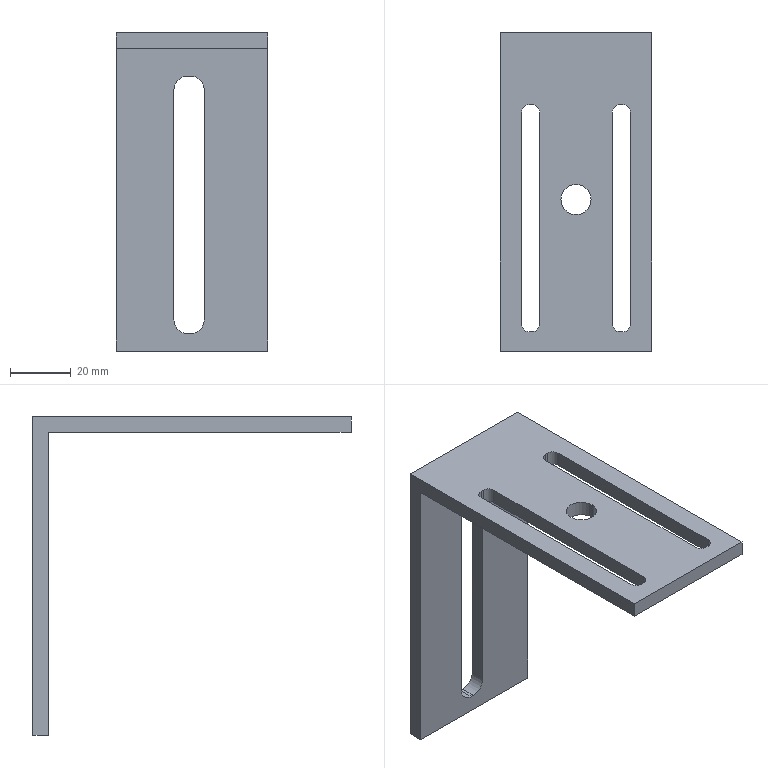Part | SolidWorks | features ICE 4, Extrusion 1 | 1 solid | 34 faces | box 50 x 105 x 105 mm | volume 42248 mm3 | plane 20 | cylinder 14 | commonest cylinder face diameters 5 x8 9 x4 10 x2
STEP:
#1=CARTESIAN_POINT('',(-5.,0.,0.));
#2=VERTEX_POINT('',#1);
#3=CARTESIAN_POINT('',(5.,0.,0.));
#4=VERTEX_POINT('',#3);
#5=CARTESIAN_POINT('',(0.,0.,0.));
#6=DIRECTION('',(0.,0.,1.));
#7=DIRECTION('',(1.,0.,0.));
#8=AXIS2_PLACEMENT_3D('',#5,#6,#7);
#9=CIRCLE('',#8,5.);
#10=EDGE_CURVE('',#2,#4,#9,.T.);
#11=ORIENTED_EDGE('',*,*,#10,.F.);
#12=CARTESIAN_POINT('',(-5.,0.,5.));
#13=VERTEX_POINT('',#12);
#14=CARTESIAN_POINT('',(-5.,0.,-5.));
#15=DIRECTION('',(0.,0.,1.));
#16=VECTOR('',#15,1000.);
#17=LINE('',#14,#16);
#18=EDGE_CURVE('',#2,#13,#17,.T.);
#19=ORIENTED_EDGE('',*,*,#18,.T.);
#20=CARTESIAN_POINT('',(5.,0.,5.));
#21=VERTEX_POINT('',#20);
#22=CARTESIAN_POINT('',(0.,0.,5.));
#23=DIRECTION('',(0.,0.,1.));
#24=DIRECTION('',(1.,0.,0.));
#25=AXIS2_PLACEMENT_3D('',#22,#23,#24);
#26=CIRCLE('',#25,5.);
#27=EDGE_CURVE('',#13,#21,#26,.T.);
#28=ORIENTED_EDGE('',*,*,#27,.T.);
#29=CARTESIAN_POINT('',(5.,0.,-5.));
#30=DIRECTION('',(0.,0.,1.));
#31=VECTOR('',#30,1000.);
#32=LINE('',#29,#31);
#33=EDGE_CURVE('',#4,#21,#32,.T.);
#34=ORIENTED_EDGE('',*,*,#33,.F.);
#35=EDGE_LOOP('',(#11,#19,#28,#34));
#36=FACE_OUTER_BOUND('',#35,.T.);
#37=CARTESIAN_POINT('',(0.,0.,-5.));
#38=DIRECTION('',(0.,0.,1.));
#39=DIRECTION('',(1.,0.,0.));
#40=AXIS2_PLACEMENT_3D('',#37,#38,#39);
#41=CYLINDRICAL_SURFACE('',#40,5.);
#42=ADVANCED_FACE('',(#36),#41,.F.);
#43=CARTESIAN_POINT('',(-25.,50.,0.));
#44=VERTEX_POINT('',#43);
#45=CARTESIAN_POINT('',(-25.,-50.,0.));
#46=VERTEX_POINT('',#45);
#47=CARTESIAN_POINT('',(-25.,-50.,0.));
#48=DIRECTION('',(0.,-1.,0.));
#49=VECTOR('',#48,1000.);
#50=LINE('',#47,#49);
#51=EDGE_CURVE('',#44,#46,#50,.T.);
#52=ORIENTED_EDGE('',*,*,#51,.T.);
#53=CARTESIAN_POINT('',(-25.,-50.,5.));
#54=VERTEX_POINT('',#53);
#55=CARTESIAN_POINT('',(-25.,-50.,5.));
#56=DIRECTION('',(0.,0.,-1.));
#57=VECTOR('',#56,1000.);
#58=LINE('',#55,#57);
#59=EDGE_CURVE('',#54,#46,#58,.T.);
#60=ORIENTED_EDGE('',*,*,#59,.F.);
#61=CARTESIAN_POINT('',(-25.,55.,5.));
#62=VERTEX_POINT('',#61);
#63=CARTESIAN_POINT('',(-25.,-50.,5.));
#64=DIRECTION('',(0.,-1.,0.));
#65=VECTOR('',#64,1000.);
#66=LINE('',#63,#65);
#67=EDGE_CURVE('',#62,#54,#66,.T.);
#68=ORIENTED_EDGE('',*,*,#67,.F.);
#69=CARTESIAN_POINT('',(-25.,55.,-100.));
#70=VERTEX_POINT('',#69);
#71=CARTESIAN_POINT('',(-25.,55.,5.));
#72=DIRECTION('',(0.,0.,-1.));
#73=VECTOR('',#72,1000.);
#74=LINE('',#71,#73);
#75=EDGE_CURVE('',#62,#70,#74,.T.);
#76=ORIENTED_EDGE('',*,*,#75,.T.);
#77=CARTESIAN_POINT('',(-25.,50.,-100.));
#78=VERTEX_POINT('',#77);
#79=CARTESIAN_POINT('',(-25.,50.,-100.));
#80=DIRECTION('',(0.,1.,0.));
#81=VECTOR('',#80,1000.);
#82=LINE('',#79,#81);
#83=EDGE_CURVE('',#78,#70,#82,.T.);
#84=ORIENTED_EDGE('',*,*,#83,.F.);
#85=CARTESIAN_POINT('',(-25.,50.,5.));
#86=DIRECTION('',(0.,0.,-1.));
#87=VECTOR('',#86,1000.);
#88=LINE('',#85,#87);
#89=EDGE_CURVE('',#44,#78,#88,.T.);
#90=ORIENTED_EDGE('',*,*,#89,.F.);
#91=EDGE_LOOP('',(#52,#60,#68,#76,#84,#90));
#92=FACE_OUTER_BOUND('',#91,.T.);
#93=CARTESIAN_POINT('',(-25.,-50.,5.));
#94=DIRECTION('',(1.,0.,0.));
#95=DIRECTION('',(0.,0.,-1.));
#96=AXIS2_PLACEMENT_3D('',#93,#94,#95);
#97=PLANE('',#96);
#98=ADVANCED_FACE('',(#92),#97,.F.);
#99=CARTESIAN_POINT('',(25.,-50.,0.));
#100=VERTEX_POINT('',#99);
#101=CARTESIAN_POINT('',(25.,-50.,0.));
#102=DIRECTION('',(1.,0.,0.));
#103=VECTOR('',#102,1000.);
#104=LINE('',#101,#103);
#105=EDGE_CURVE('',#46,#100,#104,.T.);
#106=ORIENTED_EDGE('',*,*,#105,.T.);
#107=CARTESIAN_POINT('',(25.,-50.,5.));
#108=VERTEX_POINT('',#107);
#109=CARTESIAN_POINT('',(25.,-50.,5.));
#110=DIRECTION('',(0.,0.,-1.));
#111=VECTOR('',#110,1000.);
#112=LINE('',#109,#111);
#113=EDGE_CURVE('',#108,#100,#112,.T.);
#114=ORIENTED_EDGE('',*,*,#113,.F.);
#115=CARTESIAN_POINT('',(25.,-50.,5.));
#116=DIRECTION('',(1.,0.,0.));
#117=VECTOR('',#116,1000.);
#118=LINE('',#115,#117);
#119=EDGE_CURVE('',#54,#108,#118,.T.);
#120=ORIENTED_EDGE('',*,*,#119,.F.);
#121=ORIENTED_EDGE('',*,*,#59,.T.);
#122=EDGE_LOOP('',(#106,#114,#120,#121));
#123=FACE_OUTER_BOUND('',#122,.T.);
#124=CARTESIAN_POINT('',(25.,-50.,5.));
#125=DIRECTION('',(0.,1.,0.));
#126=DIRECTION('',(-1.,0.,0.));
#127=AXIS2_PLACEMENT_3D('',#124,#125,#126);
#128=PLANE('',#127);
#129=ADVANCED_FACE('',(#123),#128,.F.);
#130=CARTESIAN_POINT('',(25.,50.,0.));
#131=VERTEX_POINT('',#130);
#132=CARTESIAN_POINT('',(25.,-50.,0.));
#133=DIRECTION('',(0.,1.,0.));
#134=VECTOR('',#133,1000.);
#135=LINE('',#132,#134);
#136=EDGE_CURVE('',#100,#131,#135,.T.);
#137=ORIENTED_EDGE('',*,*,#136,.T.);
#138=CARTESIAN_POINT('',(25.,50.,-100.));
#139=VERTEX_POINT('',#138);
#140=CARTESIAN_POINT('',(25.,50.,5.));
#141=DIRECTION('',(0.,0.,-1.));
#142=VECTOR('',#141,1000.);
#143=LINE('',#140,#142);
#144=EDGE_CURVE('',#131,#139,#143,.T.);
#145=ORIENTED_EDGE('',*,*,#144,.T.);
#146=CARTESIAN_POINT('',(25.,55.,-100.));
#147=VERTEX_POINT('',#146);
#148=CARTESIAN_POINT('',(25.,50.,-100.));
#149=DIRECTION('',(0.,-1.,0.));
#150=VECTOR('',#149,1000.);
#151=LINE('',#148,#150);
#152=EDGE_CURVE('',#147,#139,#151,.T.);
#153=ORIENTED_EDGE('',*,*,#152,.F.);
#154=CARTESIAN_POINT('',(25.,55.,5.));
#155=VERTEX_POINT('',#154);
#156=CARTESIAN_POINT('',(25.,55.,5.));
#157=DIRECTION('',(0.,0.,-1.));
#158=VECTOR('',#157,1000.);
#159=LINE('',#156,#158);
#160=EDGE_CURVE('',#155,#147,#159,.T.);
#161=ORIENTED_EDGE('',*,*,#160,.F.);
#162=CARTESIAN_POINT('',(25.,-50.,5.));
#163=DIRECTION('',(0.,1.,0.));
#164=VECTOR('',#163,1000.);
#165=LINE('',#162,#164);
#166=EDGE_CURVE('',#108,#155,#165,.T.);
#167=ORIENTED_EDGE('',*,*,#166,.F.);
#168=ORIENTED_EDGE('',*,*,#113,.T.);
#169=EDGE_LOOP('',(#137,#145,#153,#161,#167,#168));
#170=FACE_OUTER_BOUND('',#169,.T.);
#171=CARTESIAN_POINT('',(25.,-50.,5.));
#172=DIRECTION('',(-1.,0.,0.));
#173=DIRECTION('',(0.,0.,1.));
#174=AXIS2_PLACEMENT_3D('',#171,#172,#173);
#175=PLANE('',#174);
#176=ADVANCED_FACE('',(#170),#175,.F.);
#177=CARTESIAN_POINT('',(0.,0.,5.));
#178=DIRECTION('',(0.,0.,1.));
#179=DIRECTION('',(1.,0.,0.));
#180=AXIS2_PLACEMENT_3D('',#177,#178,#179);
#181=CIRCLE('',#180,5.);
#182=EDGE_CURVE('',#21,#13,#181,.T.);
#183=ORIENTED_EDGE('',*,*,#182,.F.);
#184=ORIENTED_EDGE('',*,*,#27,.F.);
#185=EDGE_LOOP('',(#183,#184));
#186=FACE_BOUND('',#185,.T.);
#187=CARTESIAN_POINT('',(-18.,-41.155,5.));
#188=VERTEX_POINT('',#187);
#189=CARTESIAN_POINT('',(-15.5,-43.655,5.));
#190=VERTEX_POINT('',#189);
#191=CARTESIAN_POINT('',(-15.5,-41.155,5.));
#192=DIRECTION('',(0.,0.,1.));
#193=DIRECTION('',(-1.,0.,0.));
#194=AXIS2_PLACEMENT_3D('',#191,#192,#193);
#195=CIRCLE('',#194,2.5);
#196=EDGE_CURVE('',#188,#190,#195,.T.);
#197=ORIENTED_EDGE('',*,*,#196,.F.);
#198=CARTESIAN_POINT('',(-18.,28.845,5.));
#199=VERTEX_POINT('',#198);
#200=CARTESIAN_POINT('',(-18.,-41.155,5.));
#201=DIRECTION('',(0.,-1.,0.));
#202=VECTOR('',#201,1000.);
#203=LINE('',#200,#202);
#204=EDGE_CURVE('',#199,#188,#203,.T.);
#205=ORIENTED_EDGE('',*,*,#204,.F.);
#206=CARTESIAN_POINT('',(-15.5,31.345,5.));
#207=VERTEX_POINT('',#206);
#208=CARTESIAN_POINT('',(-15.5,28.845,5.));
#209=DIRECTION('',(0.,0.,1.));
#210=DIRECTION('',(1.,0.,0.));
#211=AXIS2_PLACEMENT_3D('',#208,#209,#210);
#212=CIRCLE('',#211,2.5);
#213=EDGE_CURVE('',#207,#199,#212,.T.);
#214=ORIENTED_EDGE('',*,*,#213,.F.);
#215=CARTESIAN_POINT('',(-14.5,31.345,5.));
#216=VERTEX_POINT('',#215);
#217=CARTESIAN_POINT('',(-14.5,31.345,5.));
#218=DIRECTION('',(-1.,0.,0.));
#219=VECTOR('',#218,1000.);
#220=LINE('',#217,#219);
#221=EDGE_CURVE('',#216,#207,#220,.T.);
#222=ORIENTED_EDGE('',*,*,#221,.F.);
#223=CARTESIAN_POINT('',(-12.,28.845,5.));
#224=VERTEX_POINT('',#223);
#225=CARTESIAN_POINT('',(-14.5,28.845,5.));
#226=DIRECTION('',(0.,0.,1.));
#227=DIRECTION('',(1.,0.,0.));
#228=AXIS2_PLACEMENT_3D('',#225,#226,#227);
#229=CIRCLE('',#228,2.5);
#230=EDGE_CURVE('',#224,#216,#229,.T.);
#231=ORIENTED_EDGE('',*,*,#230,.F.);
#232=CARTESIAN_POINT('',(-12.,-41.155,5.));
#233=VERTEX_POINT('',#232);
#234=CARTESIAN_POINT('',(-12.,-41.155,5.));
#235=DIRECTION('',(0.,1.,0.));
#236=VECTOR('',#235,1000.);
#237=LINE('',#234,#236);
#238=EDGE_CURVE('',#233,#224,#237,.T.);
#239=ORIENTED_EDGE('',*,*,#238,.F.);
#240=CARTESIAN_POINT('',(-14.5,-43.655,5.));
#241=VERTEX_POINT('',#240);
#242=CARTESIAN_POINT('',(-14.5,-41.155,5.));
#243=DIRECTION('',(0.,0.,1.));
#244=DIRECTION('',(1.,0.,0.));
#245=AXIS2_PLACEMENT_3D('',#242,#243,#244);
#246=CIRCLE('',#245,2.5);
#247=EDGE_CURVE('',#241,#233,#246,.T.);
#248=ORIENTED_EDGE('',*,*,#247,.F.);
#249=CARTESIAN_POINT('',(-14.5,-43.655,5.));
#250=DIRECTION('',(1.,0.,0.));
#251=VECTOR('',#250,1000.);
#252=LINE('',#249,#251);
#253=EDGE_CURVE('',#190,#241,#252,.T.);
#254=ORIENTED_EDGE('',*,*,#253,.F.);
#255=EDGE_LOOP('',(#197,#205,#214,#222,#231,#239,#248,#254));
#256=FACE_BOUND('',#255,.T.);
#257=CARTESIAN_POINT('',(14.5,31.345,5.));
#258=VERTEX_POINT('',#257);
#259=CARTESIAN_POINT('',(12.,28.845,5.));
#260=VERTEX_POINT('',#259);
#261=CARTESIAN_POINT('',(14.5,28.845,5.));
#262=DIRECTION('',(0.,0.,1.));
#263=DIRECTION('',(1.,0.,0.));
#264=AXIS2_PLACEMENT_3D('',#261,#262,#263);
#265=CIRCLE('',#264,2.5);
#266=EDGE_CURVE('',#258,#260,#265,.T.);
#267=ORIENTED_EDGE('',*,*,#266,.F.);
#268=CARTESIAN_POINT('',(15.5,31.345,5.));
#269=VERTEX_POINT('',#268);
#270=CARTESIAN_POINT('',(15.5,31.345,5.));
#271=DIRECTION('',(-1.,0.,0.));
#272=VECTOR('',#271,1000.);
#273=LINE('',#270,#272);
#274=EDGE_CURVE('',#269,#258,#273,.T.);
#275=ORIENTED_EDGE('',*,*,#274,.F.);
#276=CARTESIAN_POINT('',(18.,28.845,5.));
#277=VERTEX_POINT('',#276);
#278=CARTESIAN_POINT('',(15.5,28.845,5.));
#279=DIRECTION('',(0.,0.,1.));
#280=DIRECTION('',(1.,0.,0.));
#281=AXIS2_PLACEMENT_3D('',#278,#279,#280);
#282=CIRCLE('',#281,2.5);
#283=EDGE_CURVE('',#277,#269,#282,.T.);
#284=ORIENTED_EDGE('',*,*,#283,.F.);
#285=CARTESIAN_POINT('',(18.,-41.155,5.));
#286=VERTEX_POINT('',#285);
#287=CARTESIAN_POINT('',(18.,-41.155,5.));
#288=DIRECTION('',(0.,1.,0.));
#289=VECTOR('',#288,1000.);
#290=LINE('',#287,#289);
#291=EDGE_CURVE('',#286,#277,#290,.T.);
#292=ORIENTED_EDGE('',*,*,#291,.F.);
#293=CARTESIAN_POINT('',(15.5,-43.655,5.));
#294=VERTEX_POINT('',#293);
#295=CARTESIAN_POINT('',(15.5,-41.155,5.));
#296=DIRECTION('',(0.,0.,1.));
#297=DIRECTION('',(1.,0.,0.));
#298=AXIS2_PLACEMENT_3D('',#295,#296,#297);
#299=CIRCLE('',#298,2.5);
#300=EDGE_CURVE('',#294,#286,#299,.T.);
#301=ORIENTED_EDGE('',*,*,#300,.F.);
#302=CARTESIAN_POINT('',(14.5,-43.655,5.));
#303=VERTEX_POINT('',#302);
#304=CARTESIAN_POINT('',(15.5,-43.655,5.));
#305=DIRECTION('',(1.,0.,0.));
#306=VECTOR('',#305,1000.);
#307=LINE('',#304,#306);
#308=EDGE_CURVE('',#303,#294,#307,.T.);
#309=ORIENTED_EDGE('',*,*,#308,.F.);
#310=CARTESIAN_POINT('',(12.,-41.155,5.));
#311=VERTEX_POINT('',#310);
#312=CARTESIAN_POINT('',(14.5,-41.155,5.));
#313=DIRECTION('',(0.,0.,1.));
#314=DIRECTION('',(-1.,0.,0.));
#315=AXIS2_PLACEMENT_3D('',#312,#313,#314);
#316=CIRCLE('',#315,2.5);
#317=EDGE_CURVE('',#311,#303,#316,.T.);
#318=ORIENTED_EDGE('',*,*,#317,.F.);
#319=CARTESIAN_POINT('',(12.,-41.155,5.));
#320=DIRECTION('',(0.,-1.,0.));
#321=VECTOR('',#320,1000.);
#322=LINE('',#319,#321);
#323=EDGE_CURVE('',#260,#311,#322,.T.);
#324=ORIENTED_EDGE('',*,*,#323,.F.);
#325=EDGE_LOOP('',(#267,#275,#284,#292,#301,#309,#318,#324));
#326=FACE_BOUND('',#325,.T.);
#327=ORIENTED_EDGE('',*,*,#67,.T.);
#328=ORIENTED_EDGE('',*,*,#119,.T.);
#329=ORIENTED_EDGE('',*,*,#166,.T.);
#330=CARTESIAN_POINT('',(-25.,55.,5.));
#331=DIRECTION('',(1.,0.,0.));
#332=VECTOR('',#331,1000.);
#333=LINE('',#330,#332);
#334=EDGE_CURVE('',#62,#155,#333,.T.);
#335=ORIENTED_EDGE('',*,*,#334,.F.);
#336=EDGE_LOOP('',(#327,#328,#329,#335));
#337=FACE_OUTER_BOUND('',#336,.T.);
#338=CARTESIAN_POINT('',(-25.,50.,5.));
#339=DIRECTION('',(0.,0.,1.));
#340=DIRECTION('',(1.,0.,0.));
#341=AXIS2_PLACEMENT_3D('',#338,#339,#340);
#342=PLANE('',#341);
#343=ADVANCED_FACE('',(#186,#256,#326,#337),#342,.T.);
#344=CARTESIAN_POINT('',(0.,0.,0.));
#345=DIRECTION('',(0.,0.,1.));
#346=DIRECTION('',(1.,0.,0.));
#347=AXIS2_PLACEMENT_3D('',#344,#345,#346);
#348=CIRCLE('',#347,5.);
#349=EDGE_CURVE('',#4,#2,#348,.T.);
#350=ORIENTED_EDGE('',*,*,#349,.T.);
#351=ORIENTED_EDGE('',*,*,#10,.T.);
#352=EDGE_LOOP('',(#350,#351));
#353=FACE_BOUND('',#352,.T.);
#354=CARTESIAN_POINT('',(-18.,28.845,0.));
#355=VERTEX_POINT('',#354);
#356=CARTESIAN_POINT('',(-18.,-41.155,0.));
#357=VERTEX_POINT('',#356);
#358=CARTESIAN_POINT('',(-18.,50.,0.));
#359=DIRECTION('',(0.,-1.,0.));
#360=VECTOR('',#359,1000.);
#361=LINE('',#358,#360);
#362=EDGE_CURVE('',#355,#357,#361,.T.);
#363=ORIENTED_EDGE('',*,*,#362,.T.);
#364=CARTESIAN_POINT('',(-15.5,-43.655,0.));
#365=VERTEX_POINT('',#364);
#366=CARTESIAN_POINT('',(-15.5,-41.155,0.));
#367=DIRECTION('',(0.,0.,1.));
#368=DIRECTION('',(1.,0.,0.));
#369=AXIS2_PLACEMENT_3D('',#366,#367,#368);
#370=CIRCLE('',#369,2.5);
#371=EDGE_CURVE('',#357,#365,#370,.T.);
#372=ORIENTED_EDGE('',*,*,#371,.T.);
#373=CARTESIAN_POINT('',(-14.5,-43.655,0.));
#374=VERTEX_POINT('',#373);
#375=CARTESIAN_POINT('',(-25.,-43.655,0.));
#376=DIRECTION('',(1.,0.,0.));
#377=VECTOR('',#376,1000.);
#378=LINE('',#375,#377);
#379=EDGE_CURVE('',#365,#374,#378,.T.);
#380=ORIENTED_EDGE('',*,*,#379,.T.);
#381=CARTESIAN_POINT('',(-12.,-41.155,0.));
#382=VERTEX_POINT('',#381);
#383=CARTESIAN_POINT('',(-14.5,-41.155,0.));
#384=DIRECTION('',(0.,0.,1.));
#385=DIRECTION('',(1.,0.,0.));
#386=AXIS2_PLACEMENT_3D('',#383,#384,#385);
#387=CIRCLE('',#386,2.5);
#388=EDGE_CURVE('',#374,#382,#387,.T.);
#389=ORIENTED_EDGE('',*,*,#388,.T.);
#390=CARTESIAN_POINT('',(-12.,28.845,0.));
#391=VERTEX_POINT('',#390);
#392=CARTESIAN_POINT('',(-12.,50.,0.));
#393=DIRECTION('',(0.,1.,0.));
#394=VECTOR('',#393,1000.);
#395=LINE('',#392,#394);
#396=EDGE_CURVE('',#382,#391,#395,.T.);
#397=ORIENTED_EDGE('',*,*,#396,.T.);
#398=CARTESIAN_POINT('',(-14.5,31.345,0.));
#399=VERTEX_POINT('',#398);
#400=CARTESIAN_POINT('',(-14.5,28.845,0.));
#401=DIRECTION('',(0.,0.,1.));
#402=DIRECTION('',(1.,0.,0.));
#403=AXIS2_PLACEMENT_3D('',#400,#401,#402);
#404=CIRCLE('',#403,2.5);
#405=EDGE_CURVE('',#391,#399,#404,.T.);
#406=ORIENTED_EDGE('',*,*,#405,.T.);
#407=CARTESIAN_POINT('',(-15.5,31.345,0.));
#408=VERTEX_POINT('',#407);
#409=CARTESIAN_POINT('',(-25.,31.345,0.));
#410=DIRECTION('',(-1.,0.,0.));
#411=VECTOR('',#410,1000.);
#412=LINE('',#409,#411);
#413=EDGE_CURVE('',#399,#408,#412,.T.);
#414=ORIENTED_EDGE('',*,*,#413,.T.);
#415=CARTESIAN_POINT('',(-15.5,28.845,0.));
#416=DIRECTION('',(0.,0.,1.));
#417=DIRECTION('',(1.,0.,0.));
#418=AXIS2_PLACEMENT_3D('',#415,#416,#417);
#419=CIRCLE('',#418,2.5);
#420=EDGE_CURVE('',#408,#355,#419,.T.);
#421=ORIENTED_EDGE('',*,*,#420,.T.);
#422=EDGE_LOOP('',(#363,#372,#380,#389,#397,#406,#414,#421));
#423=FACE_BOUND('',#422,.T.);
#424=CARTESIAN_POINT('',(15.5,31.345,0.));
#425=VERTEX_POINT('',#424);
#426=CARTESIAN_POINT('',(14.5,31.345,0.));
#427=VERTEX_POINT('',#426);
#428=CARTESIAN_POINT('',(-25.,31.345,0.));
#429=DIRECTION('',(-1.,0.,0.));
#430=VECTOR('',#429,1000.);
#431=LINE('',#428,#430);
#432=EDGE_CURVE('',#425,#427,#431,.T.);
#433=ORIENTED_EDGE('',*,*,#432,.T.);
#434=CARTESIAN_POINT('',(12.,28.845,0.));
#435=VERTEX_POINT('',#434);
#436=CARTESIAN_POINT('',(14.5,28.845,0.));
#437=DIRECTION('',(0.,0.,1.));
#438=DIRECTION('',(1.,0.,0.));
#439=AXIS2_PLACEMENT_3D('',#436,#437,#438);
#440=CIRCLE('',#439,2.5);
#441=EDGE_CURVE('',#427,#435,#440,.T.);
#442=ORIENTED_EDGE('',*,*,#441,.T.);
#443=CARTESIAN_POINT('',(12.,-41.155,0.));
#444=VERTEX_POINT('',#443);
#445=CARTESIAN_POINT('',(12.,50.,0.));
#446=DIRECTION('',(0.,-1.,0.));
#447=VECTOR('',#446,1000.);
#448=LINE('',#445,#447);
#449=EDGE_CURVE('',#435,#444,#448,.T.);
#450=ORIENTED_EDGE('',*,*,#449,.T.);
#451=CARTESIAN_POINT('',(14.5,-43.655,0.));
#452=VERTEX_POINT('',#451);
#453=CARTESIAN_POINT('',(14.5,-41.155,0.));
#454=DIRECTION('',(0.,0.,1.));
#455=DIRECTION('',(1.,0.,0.));
#456=AXIS2_PLACEMENT_3D('',#453,#454,#455);
#457=CIRCLE('',#456,2.5);
#458=EDGE_CURVE('',#444,#452,#457,.T.);
#459=ORIENTED_EDGE('',*,*,#458,.T.);
#460=CARTESIAN_POINT('',(15.5,-43.655,0.));
#461=VERTEX_POINT('',#460);
#462=CARTESIAN_POINT('',(-25.,-43.655,0.));
#463=DIRECTION('',(1.,0.,0.));
#464=VECTOR('',#463,1000.);
#465=LINE('',#462,#464);
#466=EDGE_CURVE('',#452,#461,#465,.T.);
#467=ORIENTED_EDGE('',*,*,#466,.T.);
#468=CARTESIAN_POINT('',(18.,-41.155,0.));
#469=VERTEX_POINT('',#468);
#470=CARTESIAN_POINT('',(15.5,-41.155,0.));
#471=DIRECTION('',(0.,0.,1.));
#472=DIRECTION('',(1.,0.,0.));
#473=AXIS2_PLACEMENT_3D('',#470,#471,#472);
#474=CIRCLE('',#473,2.5);
#475=EDGE_CURVE('',#461,#469,#474,.T.);
#476=ORIENTED_EDGE('',*,*,#475,.T.);
#477=CARTESIAN_POINT('',(18.,28.845,0.));
#478=VERTEX_POINT('',#477);
#479=CARTESIAN_POINT('',(18.,50.,0.));
#480=DIRECTION('',(0.,1.,0.));
#481=VECTOR('',#480,1000.);
#482=LINE('',#479,#481);
#483=EDGE_CURVE('',#469,#478,#482,.T.);
#484=ORIENTED_EDGE('',*,*,#483,.T.);
#485=CARTESIAN_POINT('',(15.5,28.845,0.));
#486=DIRECTION('',(0.,0.,1.));
#487=DIRECTION('',(1.,0.,0.));
#488=AXIS2_PLACEMENT_3D('',#485,#486,#487);
#489=CIRCLE('',#488,2.5);
#490=EDGE_CURVE('',#478,#425,#489,.T.);
#491=ORIENTED_EDGE('',*,*,#490,.T.);
#492=EDGE_LOOP('',(#433,#442,#450,#459,#467,#476,#484,#491));
#493=FACE_BOUND('',#492,.T.);
#494=ORIENTED_EDGE('',*,*,#51,.F.);
#495=CARTESIAN_POINT('',(25.,50.,0.));
#496=DIRECTION('',(-1.,0.,0.));
#497=VECTOR('',#496,1000.);
#498=LINE('',#495,#497);
#499=EDGE_CURVE('',#131,#44,#498,.T.);
#500=ORIENTED_EDGE('',*,*,#499,.F.);
#501=ORIENTED_EDGE('',*,*,#136,.F.);
#502=ORIENTED_EDGE('',*,*,#105,.F.);
#503=EDGE_LOOP('',(#494,#500,#501,#502));
#504=FACE_OUTER_BOUND('',#503,.T.);
#505=CARTESIAN_POINT('',(-25.,50.,0.));
#506=DIRECTION('',(0.,0.,1.));
#507=DIRECTION('',(1.,0.,0.));
#508=AXIS2_PLACEMENT_3D('',#505,#506,#507);
#509=PLANE('',#508);
#510=ADVANCED_FACE('',(#353,#423,#493,#504),#509,.F.);
#511=CARTESIAN_POINT('',(14.5,31.345,-5.));
#512=DIRECTION('',(0.,0.,1.));
#513=VECTOR('',#512,1000.);
#514=LINE('',#511,#513);
#515=EDGE_CURVE('',#427,#258,#514,.T.);
#516=ORIENTED_EDGE('',*,*,#515,.T.);
#517=ORIENTED_EDGE('',*,*,#266,.T.);
#518=CARTESIAN_POINT('',(12.,28.845,-5.));
#519=DIRECTION('',(0.,0.,1.));
#520=VECTOR('',#519,1000.);
#521=LINE('',#518,#520);
#522=EDGE_CURVE('',#435,#260,#521,.T.);
#523=ORIENTED_EDGE('',*,*,#522,.F.);
#524=ORIENTED_EDGE('',*,*,#441,.F.);
#525=EDGE_LOOP('',(#516,#517,#523,#524));
#526=FACE_OUTER_BOUND('',#525,.T.);
#527=CARTESIAN_POINT('',(14.5,28.845,-5.));
#528=DIRECTION('',(0.,0.,1.));
#529=DIRECTION('',(1.,0.,0.));
#530=AXIS2_PLACEMENT_3D('',#527,#528,#529);
#531=CYLINDRICAL_SURFACE('',#530,2.5);
#532=ADVANCED_FACE('',(#526),#531,.F.);
#533=CARTESIAN_POINT('',(15.5,31.345,-5.));
#534=DIRECTION('',(0.,0.,1.));
#535=VECTOR('',#534,1000.);
#536=LINE('',#533,#535);
#537=EDGE_CURVE('',#425,#269,#536,.T.);
#538=ORIENTED_EDGE('',*,*,#537,.T.);
#539=ORIENTED_EDGE('',*,*,#274,.T.);
#540=ORIENTED_EDGE('',*,*,#515,.F.);
#541=ORIENTED_EDGE('',*,*,#432,.F.);
#542=EDGE_LOOP('',(#538,#539,#540,#541));
#543=FACE_OUTER_BOUND('',#542,.T.);
#544=CARTESIAN_POINT('',(15.5,31.345,-5.));
#545=DIRECTION('',(0.,1.,0.));
#546=DIRECTION('',(0.,0.,1.));
#547=AXIS2_PLACEMENT_3D('',#544,#545,#546);
#548=PLANE('',#547);
#549=ADVANCED_FACE('',(#543),#548,.F.);
#550=CARTESIAN_POINT('',(18.,28.845,-5.));
#551=DIRECTION('',(0.,0.,1.));
#552=VECTOR('',#551,1000.);
#553=LINE('',#550,#552);
#554=EDGE_CURVE('',#478,#277,#553,.T.);
#555=ORIENTED_EDGE('',*,*,#554,.T.);
#556=ORIENTED_EDGE('',*,*,#283,.T.);
#557=ORIENTED_EDGE('',*,*,#537,.F.);
#558=ORIENTED_EDGE('',*,*,#490,.F.);
#559=EDGE_LOOP('',(#555,#556,#557,#558));
#560=FACE_OUTER_BOUND('',#559,.T.);
#561=CARTESIAN_POINT('',(15.5,28.845,-5.));
#562=DIRECTION('',(0.,0.,1.));
#563=DIRECTION('',(1.,0.,0.));
#564=AXIS2_PLACEMENT_3D('',#561,#562,#563);
#565=CYLINDRICAL_SURFACE('',#564,2.5);
#566=ADVANCED_FACE('',(#560),#565,.F.);
#567=CARTESIAN_POINT('',(18.,-41.155,-5.));
#568=DIRECTION('',(0.,0.,1.));
#569=VECTOR('',#568,1000.);
#570=LINE('',#567,#569);
#571=EDGE_CURVE('',#469,#286,#570,.T.);
#572=ORIENTED_EDGE('',*,*,#571,.T.);
#573=ORIENTED_EDGE('',*,*,#291,.T.);
#574=ORIENTED_EDGE('',*,*,#554,.F.);
#575=ORIENTED_EDGE('',*,*,#483,.F.);
#576=EDGE_LOOP('',(#572,#573,#574,#575));
#577=FACE_OUTER_BOUND('',#576,.T.);
#578=CARTESIAN_POINT('',(18.,-41.155,-5.));
#579=DIRECTION('',(1.,0.,0.));
#580=DIRECTION('',(0.,0.,-1.));
#581=AXIS2_PLACEMENT_3D('',#578,#579,#580);
#582=PLANE('',#581);
#583=ADVANCED_FACE('',(#577),#582,.F.);
#584=CARTESIAN_POINT('',(15.5,-43.655,-5.));
#585=DIRECTION('',(0.,0.,1.));
#586=VECTOR('',#585,1000.);
#587=LINE('',#584,#586);
#588=EDGE_CURVE('',#461,#294,#587,.T.);
#589=ORIENTED_EDGE('',*,*,#588,.T.);
#590=ORIENTED_EDGE('',*,*,#300,.T.);
#591=ORIENTED_EDGE('',*,*,#571,.F.);
#592=ORIENTED_EDGE('',*,*,#475,.F.);
#593=EDGE_LOOP('',(#589,#590,#591,#592));
#594=FACE_OUTER_BOUND('',#593,.T.);
#595=CARTESIAN_POINT('',(15.5,-41.155,-5.));
#596=DIRECTION('',(0.,0.,1.));
#597=DIRECTION('',(1.,0.,0.));
#598=AXIS2_PLACEMENT_3D('',#595,#596,#597);
#599=CYLINDRICAL_SURFACE('',#598,2.5);
#600=ADVANCED_FACE('',(#594),#599,.F.);
#601=CARTESIAN_POINT('',(14.5,-43.655,-5.));
#602=DIRECTION('',(0.,0.,1.));
#603=VECTOR('',#602,1000.);
#604=LINE('',#601,#603);
#605=EDGE_CURVE('',#452,#303,#604,.T.);
#606=ORIENTED_EDGE('',*,*,#605,.T.);
#607=ORIENTED_EDGE('',*,*,#308,.T.);
#608=ORIENTED_EDGE('',*,*,#588,.F.);
#609=ORIENTED_EDGE('',*,*,#466,.F.);
#610=EDGE_LOOP('',(#606,#607,#608,#609));
#611=FACE_OUTER_BOUND('',#610,.T.);
#612=CARTESIAN_POINT('',(15.5,-43.655,-5.));
#613=DIRECTION('',(0.,-1.,0.));
#614=DIRECTION('',(0.,0.,-1.));
#615=AXIS2_PLACEMENT_3D('',#612,#613,#614);
#616=PLANE('',#615);
#617=ADVANCED_FACE('',(#611),#616,.F.);
#618=CARTESIAN_POINT('',(12.,-41.155,-5.));
#619=DIRECTION('',(0.,0.,1.));
#620=VECTOR('',#619,1000.);
#621=LINE('',#618,#620);
#622=EDGE_CURVE('',#444,#311,#621,.T.);
#623=ORIENTED_EDGE('',*,*,#622,.T.);
#624=ORIENTED_EDGE('',*,*,#317,.T.);
#625=ORIENTED_EDGE('',*,*,#605,.F.);
#626=ORIENTED_EDGE('',*,*,#458,.F.);
#627=EDGE_LOOP('',(#623,#624,#625,#626));
#628=FACE_OUTER_BOUND('',#627,.T.);
#629=CARTESIAN_POINT('',(14.5,-41.155,-5.));
#630=DIRECTION('',(0.,0.,1.));
#631=DIRECTION('',(1.,0.,0.));
#632=AXIS2_PLACEMENT_3D('',#629,#630,#631);
#633=CYLINDRICAL_SURFACE('',#632,2.5);
#634=ADVANCED_FACE('',(#628),#633,.F.);
#635=ORIENTED_EDGE('',*,*,#522,.T.);
#636=ORIENTED_EDGE('',*,*,#323,.T.);
#637=ORIENTED_EDGE('',*,*,#622,.F.);
#638=ORIENTED_EDGE('',*,*,#449,.F.);
#639=EDGE_LOOP('',(#635,#636,#637,#638));
#640=FACE_OUTER_BOUND('',#639,.T.);
#641=CARTESIAN_POINT('',(12.,-41.155,-5.));
#642=DIRECTION('',(-1.,0.,0.));
#643=DIRECTION('',(0.,0.,1.));
#644=AXIS2_PLACEMENT_3D('',#641,#642,#643);
#645=PLANE('',#644);
#646=ADVANCED_FACE('',(#640),#645,.F.);
#647=CARTESIAN_POINT('',(-18.,-41.155,-5.));
#648=DIRECTION('',(0.,0.,1.));
#649=VECTOR('',#648,1000.);
#650=LINE('',#647,#649);
#651=EDGE_CURVE('',#357,#188,#650,.T.);
#652=ORIENTED_EDGE('',*,*,#651,.T.);
#653=ORIENTED_EDGE('',*,*,#196,.T.);
#654=CARTESIAN_POINT('',(-15.5,-43.655,-5.));
#655=DIRECTION('',(0.,0.,1.));
#656=VECTOR('',#655,1000.);
#657=LINE('',#654,#656);
#658=EDGE_CURVE('',#365,#190,#657,.T.);
#659=ORIENTED_EDGE('',*,*,#658,.F.);
#660=ORIENTED_EDGE('',*,*,#371,.F.);
#661=EDGE_LOOP('',(#652,#653,#659,#660));
#662=FACE_OUTER_BOUND('',#661,.T.);
#663=CARTESIAN_POINT('',(-15.5,-41.155,-5.));
#664=DIRECTION('',(0.,0.,1.));
#665=DIRECTION('',(1.,0.,0.));
#666=AXIS2_PLACEMENT_3D('',#663,#664,#665);
#667=CYLINDRICAL_SURFACE('',#666,2.5);
#668=ADVANCED_FACE('',(#662),#667,.F.);
#669=CARTESIAN_POINT('',(-18.,28.845,-5.));
#670=DIRECTION('',(0.,0.,1.));
#671=VECTOR('',#670,1000.);
#672=LINE('',#669,#671);
#673=EDGE_CURVE('',#355,#199,#672,.T.);
#674=ORIENTED_EDGE('',*,*,#673,.T.);
#675=ORIENTED_EDGE('',*,*,#204,.T.);
#676=ORIENTED_EDGE('',*,*,#651,.F.);
#677=ORIENTED_EDGE('',*,*,#362,.F.);
#678=EDGE_LOOP('',(#674,#675,#676,#677));
#679=FACE_OUTER_BOUND('',#678,.T.);
#680=CARTESIAN_POINT('',(-18.,-41.155,-5.));
#681=DIRECTION('',(-1.,0.,0.));
#682=DIRECTION('',(0.,0.,1.));
#683=AXIS2_PLACEMENT_3D('',#680,#681,#682);
#684=PLANE('',#683);
#685=ADVANCED_FACE('',(#679),#684,.F.);
#686=CARTESIAN_POINT('',(-15.5,31.345,-5.));
#687=DIRECTION('',(0.,0.,1.));
#688=VECTOR('',#687,1000.);
#689=LINE('',#686,#688);
#690=EDGE_CURVE('',#408,#207,#689,.T.);
#691=ORIENTED_EDGE('',*,*,#690,.T.);
#692=ORIENTED_EDGE('',*,*,#213,.T.);
#693=ORIENTED_EDGE('',*,*,#673,.F.);
#694=ORIENTED_EDGE('',*,*,#420,.F.);
#695=EDGE_LOOP('',(#691,#692,#693,#694));
#696=FACE_OUTER_BOUND('',#695,.T.);
#697=CARTESIAN_POINT('',(-15.5,28.845,-5.));
#698=DIRECTION('',(0.,0.,1.));
#699=DIRECTION('',(1.,0.,0.));
#700=AXIS2_PLACEMENT_3D('',#697,#698,#699);
#701=CYLINDRICAL_SURFACE('',#700,2.5);
#702=ADVANCED_FACE('',(#696),#701,.F.);
#703=CARTESIAN_POINT('',(-14.5,31.345,-5.));
#704=DIRECTION('',(0.,0.,1.));
#705=VECTOR('',#704,1000.);
#706=LINE('',#703,#705);
#707=EDGE_CURVE('',#399,#216,#706,.T.);
#708=ORIENTED_EDGE('',*,*,#707,.T.);
#709=ORIENTED_EDGE('',*,*,#221,.T.);
#710=ORIENTED_EDGE('',*,*,#690,.F.);
#711=ORIENTED_EDGE('',*,*,#413,.F.);
#712=EDGE_LOOP('',(#708,#709,#710,#711));
#713=FACE_OUTER_BOUND('',#712,.T.);
#714=CARTESIAN_POINT('',(-14.5,31.345,-5.));
#715=DIRECTION('',(0.,1.,0.));
#716=DIRECTION('',(0.,0.,1.));
#717=AXIS2_PLACEMENT_3D('',#714,#715,#716);
#718=PLANE('',#717);
#719=ADVANCED_FACE('',(#713),#718,.F.);
#720=CARTESIAN_POINT('',(-12.,28.845,-5.));
#721=DIRECTION('',(0.,0.,1.));
#722=VECTOR('',#721,1000.);
#723=LINE('',#720,#722);
#724=EDGE_CURVE('',#391,#224,#723,.T.);
#725=ORIENTED_EDGE('',*,*,#724,.T.);
#726=ORIENTED_EDGE('',*,*,#230,.T.);
#727=ORIENTED_EDGE('',*,*,#707,.F.);
#728=ORIENTED_EDGE('',*,*,#405,.F.);
#729=EDGE_LOOP('',(#725,#726,#727,#728));
#730=FACE_OUTER_BOUND('',#729,.T.);
#731=CARTESIAN_POINT('',(-14.5,28.845,-5.));
#732=DIRECTION('',(0.,0.,1.));
#733=DIRECTION('',(1.,0.,0.));
#734=AXIS2_PLACEMENT_3D('',#731,#732,#733);
#735=CYLINDRICAL_SURFACE('',#734,2.5);
#736=ADVANCED_FACE('',(#730),#735,.F.);
#737=CARTESIAN_POINT('',(-12.,-41.155,-5.));
#738=DIRECTION('',(0.,0.,1.));
#739=VECTOR('',#738,1000.);
#740=LINE('',#737,#739);
#741=EDGE_CURVE('',#382,#233,#740,.T.);
#742=ORIENTED_EDGE('',*,*,#741,.T.);
#743=ORIENTED_EDGE('',*,*,#238,.T.);
#744=ORIENTED_EDGE('',*,*,#724,.F.);
#745=ORIENTED_EDGE('',*,*,#396,.F.);
#746=EDGE_LOOP('',(#742,#743,#744,#745));
#747=FACE_OUTER_BOUND('',#746,.T.);
#748=CARTESIAN_POINT('',(-12.,-41.155,-5.));
#749=DIRECTION('',(1.,0.,0.));
#750=DIRECTION('',(0.,0.,-1.));
#751=AXIS2_PLACEMENT_3D('',#748,#749,#750);
#752=PLANE('',#751);
#753=ADVANCED_FACE('',(#747),#752,.F.);
#754=CARTESIAN_POINT('',(-14.5,-43.655,-5.));
#755=DIRECTION('',(0.,0.,1.));
#756=VECTOR('',#755,1000.);
#757=LINE('',#754,#756);
#758=EDGE_CURVE('',#374,#241,#757,.T.);
#759=ORIENTED_EDGE('',*,*,#758,.T.);
#760=ORIENTED_EDGE('',*,*,#247,.T.);
#761=ORIENTED_EDGE('',*,*,#741,.F.);
#762=ORIENTED_EDGE('',*,*,#388,.F.);
#763=EDGE_LOOP('',(#759,#760,#761,#762));
#764=FACE_OUTER_BOUND('',#763,.T.);
#765=CARTESIAN_POINT('',(-14.5,-41.155,-5.));
#766=DIRECTION('',(0.,0.,1.));
#767=DIRECTION('',(1.,0.,0.));
#768=AXIS2_PLACEMENT_3D('',#765,#766,#767);
#769=CYLINDRICAL_SURFACE('',#768,2.5);
#770=ADVANCED_FACE('',(#764),#769,.F.);
#771=ORIENTED_EDGE('',*,*,#658,.T.);
#772=ORIENTED_EDGE('',*,*,#253,.T.);
#773=ORIENTED_EDGE('',*,*,#758,.F.);
#774=ORIENTED_EDGE('',*,*,#379,.F.);
#775=EDGE_LOOP('',(#771,#772,#773,#774));
#776=FACE_OUTER_BOUND('',#775,.T.);
#777=CARTESIAN_POINT('',(-14.5,-43.655,-5.));
#778=DIRECTION('',(0.,-1.,0.));
#779=DIRECTION('',(0.,0.,-1.));
#780=AXIS2_PLACEMENT_3D('',#777,#778,#779);
#781=PLANE('',#780);
#782=ADVANCED_FACE('',(#776),#781,.F.);
#783=ORIENTED_EDGE('',*,*,#18,.F.);
#784=ORIENTED_EDGE('',*,*,#349,.F.);
#785=ORIENTED_EDGE('',*,*,#33,.T.);
#786=ORIENTED_EDGE('',*,*,#182,.T.);
#787=EDGE_LOOP('',(#783,#784,#785,#786));
#788=FACE_OUTER_BOUND('',#787,.T.);
#789=CARTESIAN_POINT('',(0.,0.,-5.));
#790=DIRECTION('',(0.,0.,1.));
#791=DIRECTION('',(1.,0.,0.));
#792=AXIS2_PLACEMENT_3D('',#789,#790,#791);
#793=CYLINDRICAL_SURFACE('',#792,5.);
#794=ADVANCED_FACE('',(#788),#793,.F.);
#795=CARTESIAN_POINT('',(-5.974,50.,-89.753));
#796=VERTEX_POINT('',#795);
#797=CARTESIAN_POINT('',(-1.474,50.,-94.253));
#798=VERTEX_POINT('',#797);
#799=CARTESIAN_POINT('',(-1.474,50.,-89.753));
#800=DIRECTION('',(0.,-1.,0.));
#801=DIRECTION('',(-1.,0.,0.));
#802=AXIS2_PLACEMENT_3D('',#799,#800,#801);
#803=CIRCLE('',#802,4.5);
#804=EDGE_CURVE('',#796,#798,#803,.T.);
#805=ORIENTED_EDGE('',*,*,#804,.F.);
#806=CARTESIAN_POINT('',(-5.974,50.,-13.753));
#807=VERTEX_POINT('',#806);
#808=CARTESIAN_POINT('',(-5.974,50.,-89.753));
#809=DIRECTION('',(0.,0.,-1.));
#810=VECTOR('',#809,1000.);
#811=LINE('',#808,#810);
#812=EDGE_CURVE('',#807,#796,#811,.T.);
#813=ORIENTED_EDGE('',*,*,#812,.F.);
#814=CARTESIAN_POINT('',(-1.474,50.,-9.253));
#815=VERTEX_POINT('',#814);
#816=CARTESIAN_POINT('',(-1.474,50.,-13.753));
#817=DIRECTION('',(0.,-1.,0.));
#818=DIRECTION('',(1.,0.,0.));
#819=AXIS2_PLACEMENT_3D('',#816,#817,#818);
#820=CIRCLE('',#819,4.5);
#821=EDGE_CURVE('',#815,#807,#820,.T.);
#822=ORIENTED_EDGE('',*,*,#821,.F.);
#823=CARTESIAN_POINT('',(-0.474,50.,-9.253));
#824=VERTEX_POINT('',#823);
#825=CARTESIAN_POINT('',(-0.474,50.,-9.253));
#826=DIRECTION('',(-1.,0.,0.));
#827=VECTOR('',#826,1000.);
#828=LINE('',#825,#827);
#829=EDGE_CURVE('',#824,#815,#828,.T.);
#830=ORIENTED_EDGE('',*,*,#829,.F.);
#831=CARTESIAN_POINT('',(4.026,50.,-13.753));
#832=VERTEX_POINT('',#831);
#833=CARTESIAN_POINT('',(-0.474,50.,-13.753));
#834=DIRECTION('',(0.,-1.,0.));
#835=DIRECTION('',(1.,0.,0.));
#836=AXIS2_PLACEMENT_3D('',#833,#834,#835);
#837=CIRCLE('',#836,4.5);
#838=EDGE_CURVE('',#832,#824,#837,.T.);
#839=ORIENTED_EDGE('',*,*,#838,.F.);
#840=CARTESIAN_POINT('',(4.026,50.,-89.753));
#841=VERTEX_POINT('',#840);
#842=CARTESIAN_POINT('',(4.026,50.,-89.753));
#843=DIRECTION('',(0.,0.,1.));
#844=VECTOR('',#843,1000.);
#845=LINE('',#842,#844);
#846=EDGE_CURVE('',#841,#832,#845,.T.);
#847=ORIENTED_EDGE('',*,*,#846,.F.);
#848=CARTESIAN_POINT('',(-0.474,50.,-94.253));
#849=VERTEX_POINT('',#848);
#850=CARTESIAN_POINT('',(-0.474,50.,-89.753));
#851=DIRECTION('',(0.,-1.,0.));
#852=DIRECTION('',(1.,0.,0.));
#853=AXIS2_PLACEMENT_3D('',#850,#851,#852);
#854=CIRCLE('',#853,4.5);
#855=EDGE_CURVE('',#849,#841,#854,.T.);
#856=ORIENTED_EDGE('',*,*,#855,.F.);
#857=CARTESIAN_POINT('',(-0.474,50.,-94.253));
#858=DIRECTION('',(1.,0.,0.));
#859=VECTOR('',#858,1000.);
#860=LINE('',#857,#859);
#861=EDGE_CURVE('',#798,#849,#860,.T.);
#862=ORIENTED_EDGE('',*,*,#861,.F.);
#863=EDGE_LOOP('',(#805,#813,#822,#830,#839,#847,#856,#862));
#864=FACE_BOUND('',#863,.T.);
#865=ORIENTED_EDGE('',*,*,#144,.F.);
#866=ORIENTED_EDGE('',*,*,#499,.T.);
#867=ORIENTED_EDGE('',*,*,#89,.T.);
#868=CARTESIAN_POINT('',(-25.,50.,-100.));
#869=DIRECTION('',(-1.,0.,0.));
#870=VECTOR('',#869,1000.);
#871=LINE('',#868,#870);
#872=EDGE_CURVE('',#139,#78,#871,.T.);
#873=ORIENTED_EDGE('',*,*,#872,.F.);
#874=EDGE_LOOP('',(#865,#866,#867,#873));
#875=FACE_OUTER_BOUND('',#874,.T.);
#876=CARTESIAN_POINT('',(-25.,50.,5.));
#877=DIRECTION('',(0.,-1.,0.));
#878=DIRECTION('',(1.,0.,0.));
#879=AXIS2_PLACEMENT_3D('',#876,#877,#878);
#880=PLANE('',#879);
#881=ADVANCED_FACE('',(#864,#875),#880,.T.);
#882=CARTESIAN_POINT('',(-1.474,55.,-94.253));
#883=VERTEX_POINT('',#882);
#884=CARTESIAN_POINT('',(-5.974,55.,-89.753));
#885=VERTEX_POINT('',#884);
#886=CARTESIAN_POINT('',(-1.474,55.,-89.753));
#887=DIRECTION('',(0.,1.,0.));
#888=DIRECTION('',(-1.,0.,0.));
#889=AXIS2_PLACEMENT_3D('',#886,#887,#888);
#890=CIRCLE('',#889,4.5);
#891=EDGE_CURVE('',#883,#885,#890,.T.);
#892=ORIENTED_EDGE('',*,*,#891,.F.);
#893=CARTESIAN_POINT('',(-0.474,55.,-94.253));
#894=VERTEX_POINT('',#893);
#895=CARTESIAN_POINT('',(-25.,55.,-94.253));
#896=DIRECTION('',(-1.,0.,0.));
#897=VECTOR('',#896,1000.);
#898=LINE('',#895,#897);
#899=EDGE_CURVE('',#894,#883,#898,.T.);
#900=ORIENTED_EDGE('',*,*,#899,.F.);
#901=CARTESIAN_POINT('',(4.026,55.,-89.753));
#902=VERTEX_POINT('',#901);
#903=CARTESIAN_POINT('',(-0.474,55.,-89.753));
#904=DIRECTION('',(0.,1.,0.));
#905=DIRECTION('',(-1.,0.,0.));
#906=AXIS2_PLACEMENT_3D('',#903,#904,#905);
#907=CIRCLE('',#906,4.5);
#908=EDGE_CURVE('',#902,#894,#907,.T.);
#909=ORIENTED_EDGE('',*,*,#908,.F.);
#910=CARTESIAN_POINT('',(4.026,55.,-13.753));
#911=VERTEX_POINT('',#910);
#912=CARTESIAN_POINT('',(4.026,55.,5.));
#913=DIRECTION('',(0.,0.,-1.));
#914=VECTOR('',#913,1000.);
#915=LINE('',#912,#914);
#916=EDGE_CURVE('',#911,#902,#915,.T.);
#917=ORIENTED_EDGE('',*,*,#916,.F.);
#918=CARTESIAN_POINT('',(-0.474,55.,-9.253));
#919=VERTEX_POINT('',#918);
#920=CARTESIAN_POINT('',(-0.474,55.,-13.753));
#921=DIRECTION('',(0.,1.,0.));
#922=DIRECTION('',(-1.,0.,0.));
#923=AXIS2_PLACEMENT_3D('',#920,#921,#922);
#924=CIRCLE('',#923,4.5);
#925=EDGE_CURVE('',#919,#911,#924,.T.);
#926=ORIENTED_EDGE('',*,*,#925,.F.);
#927=CARTESIAN_POINT('',(-1.474,55.,-9.253));
#928=VERTEX_POINT('',#927);
#929=CARTESIAN_POINT('',(-25.,55.,-9.253));
#930=DIRECTION('',(1.,0.,0.));
#931=VECTOR('',#930,1000.);
#932=LINE('',#929,#931);
#933=EDGE_CURVE('',#928,#919,#932,.T.);
#934=ORIENTED_EDGE('',*,*,#933,.F.);
#935=CARTESIAN_POINT('',(-5.974,55.,-13.753));
#936=VERTEX_POINT('',#935);
#937=CARTESIAN_POINT('',(-1.474,55.,-13.753));
#938=DIRECTION('',(0.,1.,0.));
#939=DIRECTION('',(-1.,0.,0.));
#940=AXIS2_PLACEMENT_3D('',#937,#938,#939);
#941=CIRCLE('',#940,4.5);
#942=EDGE_CURVE('',#936,#928,#941,.T.);
#943=ORIENTED_EDGE('',*,*,#942,.F.);
#944=CARTESIAN_POINT('',(-5.974,55.,5.));
#945=DIRECTION('',(0.,0.,1.));
#946=VECTOR('',#945,1000.);
#947=LINE('',#944,#946);
#948=EDGE_CURVE('',#885,#936,#947,.T.);
#949=ORIENTED_EDGE('',*,*,#948,.F.);
#950=EDGE_LOOP('',(#892,#900,#909,#917,#926,#934,#943,#949));
#951=FACE_BOUND('',#950,.T.);
#952=ORIENTED_EDGE('',*,*,#160,.T.);
#953=CARTESIAN_POINT('',(-25.,55.,-100.));
#954=DIRECTION('',(1.,0.,0.));
#955=VECTOR('',#954,1000.);
#956=LINE('',#953,#955);
#957=EDGE_CURVE('',#70,#147,#956,.T.);
#958=ORIENTED_EDGE('',*,*,#957,.F.);
#959=ORIENTED_EDGE('',*,*,#75,.F.);
#960=ORIENTED_EDGE('',*,*,#334,.T.);
#961=EDGE_LOOP('',(#952,#958,#959,#960));
#962=FACE_OUTER_BOUND('',#961,.T.);
#963=CARTESIAN_POINT('',(-25.,55.,5.));
#964=DIRECTION('',(0.,1.,0.));
#965=DIRECTION('',(-1.,0.,0.));
#966=AXIS2_PLACEMENT_3D('',#963,#964,#965);
#967=PLANE('',#966);
#968=ADVANCED_FACE('',(#951,#962),#967,.T.);
#969=ORIENTED_EDGE('',*,*,#872,.T.);
#970=ORIENTED_EDGE('',*,*,#83,.T.);
#971=ORIENTED_EDGE('',*,*,#957,.T.);
#972=ORIENTED_EDGE('',*,*,#152,.T.);
#973=EDGE_LOOP('',(#969,#970,#971,#972));
#974=FACE_OUTER_BOUND('',#973,.T.);
#975=CARTESIAN_POINT('',(25.,50.,-100.));
#976=DIRECTION('',(0.,0.,1.));
#977=DIRECTION('',(1.,0.,0.));
#978=AXIS2_PLACEMENT_3D('',#975,#976,#977);
#979=PLANE('',#978);
#980=ADVANCED_FACE('',(#974),#979,.F.);
#981=ORIENTED_EDGE('',*,*,#891,.T.);
#982=CARTESIAN_POINT('',(-5.974,130.,-89.753));
#983=DIRECTION('',(0.,-1.,0.));
#984=VECTOR('',#983,1000.);
#985=LINE('',#982,#984);
#986=EDGE_CURVE('',#885,#796,#985,.T.);
#987=ORIENTED_EDGE('',*,*,#986,.T.);
#988=ORIENTED_EDGE('',*,*,#804,.T.);
#989=CARTESIAN_POINT('',(-1.474,130.,-94.253));
#990=DIRECTION('',(0.,-1.,0.));
#991=VECTOR('',#990,1000.);
#992=LINE('',#989,#991);
#993=EDGE_CURVE('',#883,#798,#992,.T.);
#994=ORIENTED_EDGE('',*,*,#993,.F.);
#995=EDGE_LOOP('',(#981,#987,#988,#994));
#996=FACE_OUTER_BOUND('',#995,.T.);
#997=CARTESIAN_POINT('',(-1.474,130.,-89.753));
#998=DIRECTION('',(0.,-1.,0.));
#999=DIRECTION('',(1.,0.,0.));
#1000=AXIS2_PLACEMENT_3D('',#997,#998,#999);
#1001=CYLINDRICAL_SURFACE('',#1000,4.5);
#1002=ADVANCED_FACE('',(#996),#1001,.F.);
#1003=ORIENTED_EDGE('',*,*,#948,.T.);
#1004=CARTESIAN_POINT('',(-5.974,130.,-13.753));
#1005=DIRECTION('',(0.,-1.,0.));
#1006=VECTOR('',#1005,1000.);
#1007=LINE('',#1004,#1006);
#1008=EDGE_CURVE('',#936,#807,#1007,.T.);
#1009=ORIENTED_EDGE('',*,*,#1008,.T.);
#1010=ORIENTED_EDGE('',*,*,#812,.T.);
#1011=ORIENTED_EDGE('',*,*,#986,.F.);
#1012=EDGE_LOOP('',(#1003,#1009,#1010,#1011));
#1013=FACE_OUTER_BOUND('',#1012,.T.);
#1014=CARTESIAN_POINT('',(-5.974,130.,-89.753));
#1015=DIRECTION('',(-1.,0.,0.));
#1016=DIRECTION('',(0.,-1.,0.));
#1017=AXIS2_PLACEMENT_3D('',#1014,#1015,#1016);
#1018=PLANE('',#1017);
#1019=ADVANCED_FACE('',(#1013),#1018,.F.);
#1020=ORIENTED_EDGE('',*,*,#942,.T.);
#1021=CARTESIAN_POINT('',(-1.474,130.,-9.253));
#1022=DIRECTION('',(0.,-1.,0.));
#1023=VECTOR('',#1022,1000.);
#1024=LINE('',#1021,#1023);
#1025=EDGE_CURVE('',#928,#815,#1024,.T.);
#1026=ORIENTED_EDGE('',*,*,#1025,.T.);
#1027=ORIENTED_EDGE('',*,*,#821,.T.);
#1028=ORIENTED_EDGE('',*,*,#1008,.F.);
#1029=EDGE_LOOP('',(#1020,#1026,#1027,#1028));
#1030=FACE_OUTER_BOUND('',#1029,.T.);
#1031=CARTESIAN_POINT('',(-1.474,130.,-13.753));
#1032=DIRECTION('',(0.,-1.,0.));
#1033=DIRECTION('',(1.,0.,0.));
#1034=AXIS2_PLACEMENT_3D('',#1031,#1032,#1033);
#1035=CYLINDRICAL_SURFACE('',#1034,4.5);
#1036=ADVANCED_FACE('',(#1030),#1035,.F.);
#1037=ORIENTED_EDGE('',*,*,#933,.T.);
#1038=CARTESIAN_POINT('',(-0.474,130.,-9.253));
#1039=DIRECTION('',(0.,-1.,0.));
#1040=VECTOR('',#1039,1000.);
#1041=LINE('',#1038,#1040);
#1042=EDGE_CURVE('',#919,#824,#1041,.T.);
#1043=ORIENTED_EDGE('',*,*,#1042,.T.);
#1044=ORIENTED_EDGE('',*,*,#829,.T.);
#1045=ORIENTED_EDGE('',*,*,#1025,.F.);
#1046=EDGE_LOOP('',(#1037,#1043,#1044,#1045));
#1047=FACE_OUTER_BOUND('',#1046,.T.);
#1048=CARTESIAN_POINT('',(-0.474,130.,-9.253));
#1049=DIRECTION('',(0.,0.,1.));
#1050=DIRECTION('',(1.,0.,0.));
#1051=AXIS2_PLACEMENT_3D('',#1048,#1049,#1050);
#1052=PLANE('',#1051);
#1053=ADVANCED_FACE('',(#1047),#1052,.F.);
#1054=ORIENTED_EDGE('',*,*,#925,.T.);
#1055=CARTESIAN_POINT('',(4.026,130.,-13.753));
#1056=DIRECTION('',(0.,-1.,0.));
#1057=VECTOR('',#1056,1000.);
#1058=LINE('',#1055,#1057);
#1059=EDGE_CURVE('',#911,#832,#1058,.T.);
#1060=ORIENTED_EDGE('',*,*,#1059,.T.);
#1061=ORIENTED_EDGE('',*,*,#838,.T.);
#1062=ORIENTED_EDGE('',*,*,#1042,.F.);
#1063=EDGE_LOOP('',(#1054,#1060,#1061,#1062));
#1064=FACE_OUTER_BOUND('',#1063,.T.);
#1065=CARTESIAN_POINT('',(-0.474,130.,-13.753));
#1066=DIRECTION('',(0.,-1.,0.));
#1067=DIRECTION('',(1.,0.,0.));
#1068=AXIS2_PLACEMENT_3D('',#1065,#1066,#1067);
#1069=CYLINDRICAL_SURFACE('',#1068,4.5);
#1070=ADVANCED_FACE('',(#1064),#1069,.F.);
#1071=ORIENTED_EDGE('',*,*,#916,.T.);
#1072=CARTESIAN_POINT('',(4.026,130.,-89.753));
#1073=DIRECTION('',(0.,-1.,0.));
#1074=VECTOR('',#1073,1000.);
#1075=LINE('',#1072,#1074);
#1076=EDGE_CURVE('',#902,#841,#1075,.T.);
#1077=ORIENTED_EDGE('',*,*,#1076,.T.);
#1078=ORIENTED_EDGE('',*,*,#846,.T.);
#1079=ORIENTED_EDGE('',*,*,#1059,.F.);
#1080=EDGE_LOOP('',(#1071,#1077,#1078,#1079));
#1081=FACE_OUTER_BOUND('',#1080,.T.);
#1082=CARTESIAN_POINT('',(4.026,130.,-89.753));
#1083=DIRECTION('',(1.,0.,0.));
#1084=DIRECTION('',(0.,1.,0.));
#1085=AXIS2_PLACEMENT_3D('',#1082,#1083,#1084);
#1086=PLANE('',#1085);
#1087=ADVANCED_FACE('',(#1081),#1086,.F.);
#1088=ORIENTED_EDGE('',*,*,#908,.T.);
#1089=CARTESIAN_POINT('',(-0.474,130.,-94.253));
#1090=DIRECTION('',(0.,-1.,0.));
#1091=VECTOR('',#1090,1000.);
#1092=LINE('',#1089,#1091);
#1093=EDGE_CURVE('',#894,#849,#1092,.T.);
#1094=ORIENTED_EDGE('',*,*,#1093,.T.);
#1095=ORIENTED_EDGE('',*,*,#855,.T.);
#1096=ORIENTED_EDGE('',*,*,#1076,.F.);
#1097=EDGE_LOOP('',(#1088,#1094,#1095,#1096));
#1098=FACE_OUTER_BOUND('',#1097,.T.);
#1099=CARTESIAN_POINT('',(-0.474,130.,-89.753));
#1100=DIRECTION('',(0.,-1.,0.));
#1101=DIRECTION('',(1.,0.,0.));
#1102=AXIS2_PLACEMENT_3D('',#1099,#1100,#1101);
#1103=CYLINDRICAL_SURFACE('',#1102,4.5);
#1104=ADVANCED_FACE('',(#1098),#1103,.F.);
#1105=ORIENTED_EDGE('',*,*,#899,.T.);
#1106=ORIENTED_EDGE('',*,*,#993,.T.);
#1107=ORIENTED_EDGE('',*,*,#861,.T.);
#1108=ORIENTED_EDGE('',*,*,#1093,.F.);
#1109=EDGE_LOOP('',(#1105,#1106,#1107,#1108));
#1110=FACE_OUTER_BOUND('',#1109,.T.);
#1111=CARTESIAN_POINT('',(-0.474,130.,-94.253));
#1112=DIRECTION('',(0.,0.,-1.));
#1113=DIRECTION('',(-1.,0.,0.));
#1114=AXIS2_PLACEMENT_3D('',#1111,#1112,#1113);
#1115=PLANE('',#1114);
#1116=ADVANCED_FACE('',(#1110),#1115,.F.);
#1117=CLOSED_SHELL('',(#42,#98,#129,#176,#343,#510,#532,#549,#566,#583,#600,#617,#634,#646,#668,#685,#702,#719,#736,#753,#770,#782,#794,#881,#968,#980,#1002,#1019,#1036,#1053,#1070,#1087,#1104,#1116));
#1118=MANIFOLD_SOLID_BREP('',#1117);
#1119=CARTESIAN_POINT('',(0.,0.,0.));
#1120=DIRECTION('',(0.,0.,1.));
#1121=DIRECTION('',(1.,0.,0.));
#1122=AXIS2_PLACEMENT_3D('',#1119,#1120,#1121);
#1123=(LENGTH_UNIT()NAMED_UNIT(*)SI_UNIT(.MILLI.,.METRE.));
#1124=UNCERTAINTY_MEASURE_WITH_UNIT(LENGTH_MEASURE(0.00001),#1123,'','');
#1125=(NAMED_UNIT(*)PLANE_ANGLE_UNIT()SI_UNIT($,.RADIAN.));
#1126=(NAMED_UNIT(*)SI_UNIT($,.STERADIAN.)SOLID_ANGLE_UNIT());
#1127=(GEOMETRIC_REPRESENTATION_CONTEXT(3)GLOBAL_UNCERTAINTY_ASSIGNED_CONTEXT((#1124))GLOBAL_UNIT_ASSIGNED_CONTEXT((#1123,#1125,#1126))REPRESENTATION_CONTEXT('',''));
#1128=ADVANCED_BREP_SHAPE_REPRESENTATION('',(#1118,#1122),#1127);